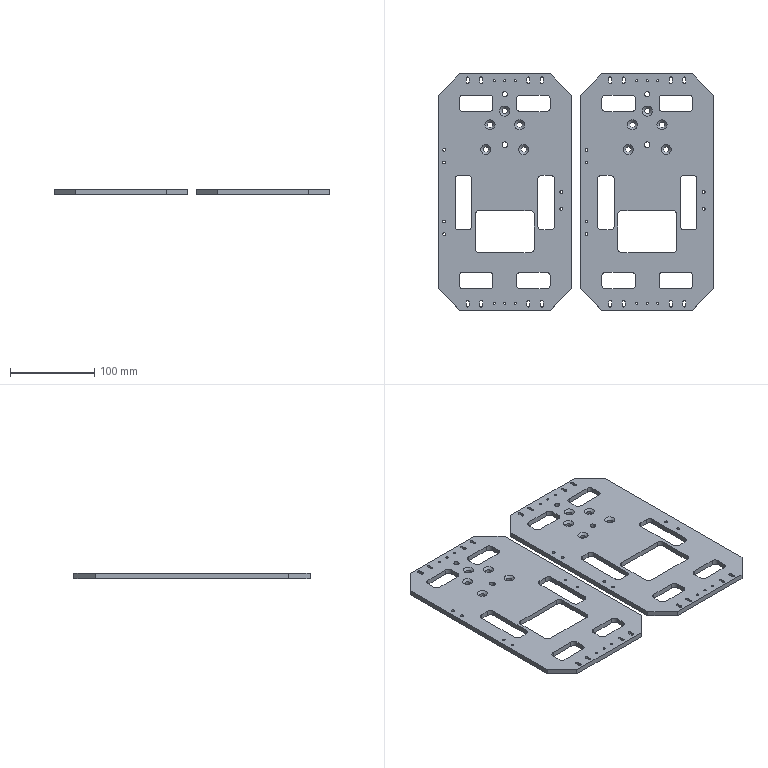CAM job | NX | 3-axis milling, drilling | part box 327 x 280 x 6 mm | stock box 332 x 285 x 6 mm
Tools:
number,name,description,diameter,corner_radius,flute_length,length,flutes
4,D4,平底铣刀-粗,4.0,0.0,25.0,75.0,2
9,D10,平底铣刀-粗,10.0,0.0,35.0,75.0,2
17,D2-J,平底铣刀-精,2.0,0.0,50.0,75.0,2
11,D4-J,平底铣刀-精,4.0,0.0,50.0,75.0,2
7,D6-J,平底铣刀-精,6.0,0.0,25.0,75.0,2
2,D6倒角刀,倒角刀,6.0,0.0,3.0,25.0,2
12,ZT2.6,钻头,2.6,0.0,35.0,50.0,2
13,ZT3.4,钻头,3.4,0.0,35.0,50.0,2
18,DRILL-BIT6.6,Drilling Tool,6.6,0.0,35.0,50.0,2
18,ZT5.9,Drilling Tool,5.9,0.0,35.0,50.0,2
Operations:
program,operation,operation_type,tool,method,geometry_group,spindle_rpm,surface_speed,feed_per_tooth,feed_cut,feed_plunge,cut_length_mm,path_length_mm,cut_time_min,machine_time_min
B,C0.3_CLOSED-CONTOUR-MILL-CHAMFER-6X45L_COPY,PlanarMilling,D6倒角刀,WALL-CLIMB_CHAMFER-DEPTH0-STEPG,W-B,7000.0,131.0,0.1071,1500.0,100.0,2303.971,5363.077,1.536,1.842
B,DRILL-CHAMFER_4,Operation,D6倒角刀,METHOD,W-B,8000.0,150.796,0.0625,1000.0,0.0,28.5,487.437,0.0285,0.0744
B,DRILL-CHAMFER_5,Operation,D6倒角刀,METHOD,W-B,8000.0,150.796,0.0625,1000.0,0.0,10.4,144.024,0.0104,0.0238
B,DRILL-CHAMFER_6,Operation,D6倒角刀,METHOD,W-B,8000.0,150.796,0.0625,1000.0,0.0,20.0,249.658,0.02,0.043
B,C0.3_CLOSED-CONTOUR-MILL-CHAMFER-6X45L_COPY_1,PlanarMilling,D6倒角刀,WALL-CLIMB_CHAMFER-DEPTH0-STEPG,W-B,7000.0,131.0,0.1071,1500.0,100.0,27.685,123.685,0.0185,0.0281
A,SPOT-POINT,Operation,D6倒角刀,METHOD,W-A,3000.0,56.549,0.0333,200.0,0.0,24.0,771.328,0.12,0.1947
A,SPOT-POINT_2,Operation,D6倒角刀,METHOD,W-A,3000.0,56.549,0.0333,200.0,0.0,60.0,1007.05,0.3,0.3947
A,HOLE-DRILL,Operation,ZT2.6,METHOD,W-A,3800.0,29.845,0.0105,80.0,0.0,78.0,879.328,0.975,1.055
A,HOLE-DRILL_2,Operation,ZT3.4,METHOD,W-A,3500.0,36.285,0.0143,100.0,0.0,26.0,324.053,0.26,0.2898
A,HOLE-DRILL_3,Operation,ZT3.4,METHOD,W-A,3000.0,32.044,0.0167,100.0,0.0,52.0,540.15,0.52,0.5688
A,HOLE-DRILL_4,Operation,ZT5.9,METHOD,W-A,3000.0,54.664,0.025,150.0,0.0,13.0,256.003,0.0867,0.111
A,HOLE-DRILL_5,Operation,DRILL-BIT6.6,METHOD,W-A,2600.0,53.91,0.0231,120.0,0.0,65.0,538.362,0.5417,0.589
A,POCKET-ROUGHING_1,VolumeBased25DMillingOperation,D10,METHOD,W-A,6000.0,188.0,0.25,4000.0,80.0,5580.614,5878.114,1.395,1.425
A,POCKET-ROUGHING_2,VolumeBased25DMillingOperation,D10,METHOD,W-A,6000.0,188.0,0.25,4000.0,80.0,7241.243,7774.047,1.81,1.864
A,POCKET-ROUGHING_3,VolumeBased25DMillingOperation,D10,METHOD,W-A,6000.0,188.0,0.25,4000.0,80.0,8882.54,10091.341,2.221,2.341
A,THROUGH-WAIST-SLOT-ROUGH_1,VolumeBased25DMillingOperation,D4,METHOD,W-A,8000.0,100.531,0.0312,500.0,100.0,1232.819,1782.2,2.466,2.521
A,WAIST-SLOT-ROUGH_1,VolumeBased25DMillingOperation,D2-J,METHOD,W-A,8000.0,50.266,0.0375,600.0,100.0,16625.796,18431.772,27.71,27.89
A,PROFILE-ROUGH_2,VolumeBased25DMillingOperation,D10,METHOD,W-A,6000.0,188.0,0.25,4000.0,80.0,22089.109,22554.309,5.522,5.569
A,POCKET-SEMI-FINISH_1,VolumeBased25DMillingOperation,D6-J,METHOD,W-A,6000.0,113.0,0.0833,1000.0,100.0,437.215,748.718,0.4372,0.4684
A,POCKET-SEMI-FINISH_2,VolumeBased25DMillingOperation,D6-J,METHOD,W-A,6000.0,113.0,0.0833,1000.0,100.0,594.43,1168.62,0.5944,0.6518
A,POCKET-SEMI-FINISH_3,VolumeBased25DMillingOperation,D6-J,METHOD,W-A,6000.0,113.0,0.0833,1000.0,100.0,788.076,2059.378,0.7881,0.9152
A,POCKET-FINISH_1,VolumeBased25DMillingOperation,D6-J,METHOD,W-A,6000.0,113.0,0.0833,1000.0,100.0,436.815,749.518,0.4368,0.4681
A,POCKET-FINISH_2,VolumeBased25DMillingOperation,D6-J,METHOD,W-A,6000.0,113.0,0.0833,1000.0,100.0,593.63,1170.387,0.5936,0.6513
A,POCKET-FINISH_3,VolumeBased25DMillingOperation,D6-J,METHOD,W-A,6000.0,113.0,0.0833,1000.0,100.0,786.575,2063.175,0.7866,0.9142
A,CONSTANT-Z-SPIRAL-WALL_COPY,ZLevelMilling,D6-J,CONSTANT-Z-WALL-DEPTHK-STEPG,W-A,7000.0,131.947,0.1429,2000.0,100.0,26462.018,27499.869,13.231,13.335
A,BOTTOM-WALL-SPIRAL-FINISH-MID_COPY_COPY_COPY_1_COPY,VolumeBased25DMillingOperation,D4-J,SPIRAL-FINISH-DEPTHK-STEPG,W-A,8000.0,50.266,0.0187,300.0,100.0,770.66,1791.179,2.569,2.671
A,BOTTOM-WALL-SPIRAL-FINISH-MID_COPY_COPY_COPY_1_COPY_COPY,VolumeBased25DMillingOperation,D2-J,SPIRAL-FINISH-DEPTHK-STEPG,W-A,8000.0,50.266,0.0187,300.0,100.0,817.094,2152.181,2.724,2.857
A,BODY-ONLY-SELECT,SurfaceContour,D6倒角刀,METHOD,W-A,6000.0,113.0,0.125,1200.0,100.0,4087.656,7521.243,3.406,3.75
A,DRILL-CHAMFER_1,Operation,D6倒角刀,METHOD,W-A,5000.0,94.248,0.015,150.0,0.0,57.0,861.919,0.38,0.4605
A,DRILL-CHAMFER_2,Operation,D6倒角刀,METHOD,W-A,5000.0,94.248,0.015,150.0,0.0,20.8,320.074,0.1387,0.1686
A,DRILL-CHAMFER_3,Operation,D6倒角刀,METHOD,W-A,5000.0,94.248,0.015,150.0,0.0,40.0,531.343,0.2667,0.3158
A,MILL-CHAMFER_1,PlanarMilling,D6倒角刀,METHOD,W-A,6000.0,113.097,0.05,600.0,100.0,37.911,330.519,0.0632,0.0924
A,WAIST-SLOT-FINISH_1,VolumeBased25DMillingOperation,D4-J,METHOD,W-A,6000.0,113.0,0.0167,200.0,100.0,76.896,677.725,0.3845,0.4446
A,WAIST-SLOT-FINISH_2,VolumeBased25DMillingOperation,D2-J,METHOD,W-A,6000.0,113.0,0.0167,200.0,100.0,1016.92,3154.325,5.085,5.298
A,PROFILE-SEMI-FINISH_2,VolumeBased25DMillingOperation,D6-J,METHOD,W-A,6000.0,113.0,0.0833,1000.0,100.0,1682.374,2228.683,1.682,1.737
A,PROFILE-FINISH_2,VolumeBased25DMillingOperation,D6-J,METHOD,W-A,6000.0,113.0,0.0833,1000.0,100.0,1681.974,2229.311,1.682,1.737